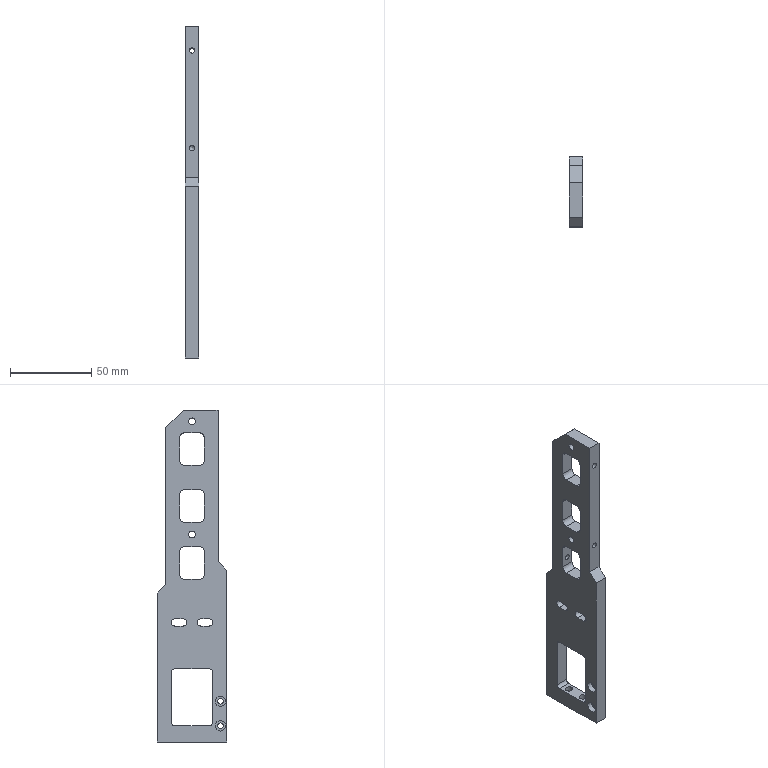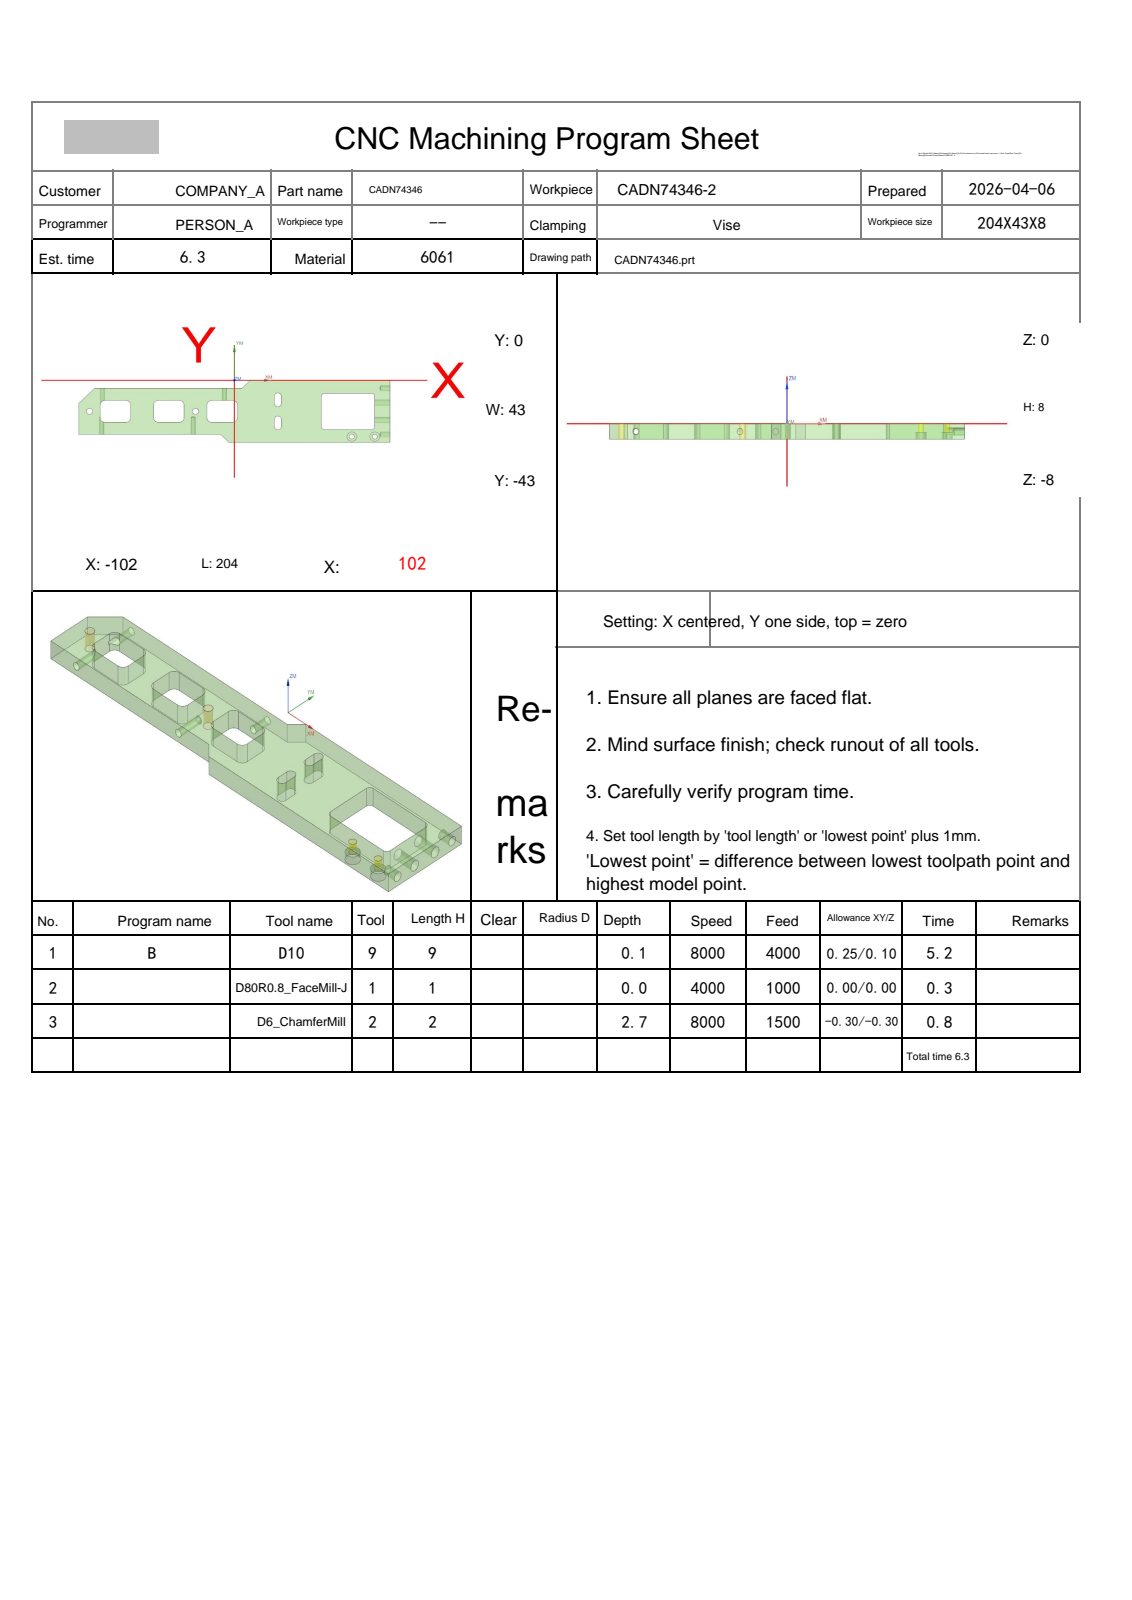NC program | NX | posted by the shop | part box 8 x 43 x 204 mm
Whole program:
%
O0001
(Machine time: 6.90 MIN)
(===Total Tool:3===)
(T9=D10     D=10.  R=0.   D-  H09 Z=0.1   )
(T1=D80R0.8 FaceMill-J D=80.  R=0.8  D-  H01 Z=0.    )
(T2=D6_ChamferMill   D=6.   R=0.   D-  H02 Z=-2.7  )
G80 G90 G17 G49 G40
G91 G28 Z0
M01
N1 T09 M06
(D10  D=10. R=0. H=09 ce=0.25 di=0.10)
G00 G90 G54 X-115.945 Y-22.484 M03 S8000
G43 H09 Z20.
M08
Z2.1
G01 X-115.846 Y-22.469 Z1.476 F4000.
X-115.747 Y-22.454 Z1.228
X-115.648 Y-22.439 Z1.046
X-115.549 Y-22.424 Z.9
X-115.45 Y-22.409 Z.777
X-115.351 Y-22.394 Z.672
X-115.252 Y-22.379 Z.58
X-115.154 Y-22.364 Z.5
X-115.055 Y-22.349 Z.43
X-114.956 Y-22.334 Z.368
X-114.857 Y-22.319 Z.314
X-114.758 Y-22.304 Z.267
X-114.659 Y-22.289 Z.227
X-114.56 Y-22.274 Z.192
X-114.462 Y-22.259 Z.164
X-114.363 Y-22.244 Z.14
X-114.264 Y-22.229 Z.123
X-114.165 Y-22.214 Z.11
X-114.066 Y-22.199 Z.103
X-113.967 Y-22.184 Z.1
X-111.744 Y-21.846
G03 X-111.332 Y-21.478 I-.079 J.502
X-110.863 Y-17.555 I-16.172 J3.923
X-110.865 Y-17.31 I-16.641 J0.0
X-110.777 Y-4.262 I-964.212 J13.048
X-110.784 Y-.447 I-964.301 J0.0
G02 X-105.871 Y6.277 I7.08 J-.016
X-100.069 Y7.207 I5.928 J-18.425
X-91.117 Y7.309 I8.952 J-392.128
X-88.92 Y7.303 I0.0 J-392.231
G01 X103.117 Y7.283
G02 X109.797 Y2.311 I-.087 J-7.089
X110.703 Y-3.395 I-18.567 J-5.872
X110.807 Y-12.349 I-384.71 J-8.954
X110.801 Y-14.594 I-384.814 J0.0
G01 X110.782 Y-42.608
G02 X105.819 Y-49.293 I-7.091 J.079
X100.062 Y-50.204 I-5.895 J18.612
X91.09 Y-50.306 I-8.972 J395.249
X88.914 Y-50.3 I0.0 J395.351
G01 X-103.206 Y-50.279
G02 X-109.795 Y-45.322 I.167 J7.081
X-110.706 Y-39.565 I18.625 J5.895
X-110.813 Y-29.529 I469.253 J10.036
X-110.769 Y-23.117 I469.361 J0.0
G03 X-110.287 Y-11.341 I-143.632 J11.776
X-110.302 Y-9.245 I-144.114 J0.0
G02 X-110.321 Y-6.601 I192.195 J2.644
X-110.247 Y-1.299 I192.213 J0.0
X-105.72 Y5.141 I7.749 J-.636
X-99.729 Y6.584 I6.779 J-14.997
X-91.153 Y6.82 I8.576 J-155.336
X-88.733 Y6.801 I0.0 J-155.573
G01 X101.703 Y6.781
G02 X108.732 Y2.029 I-.178 J-7.838
X110.114 Y-4.183 I-16.043 J-6.827
X110.322 Y-13.597 I-212.824 J-9.414
X110.3 Y-16.63 I-213.032 J0.0
G01 X110.279 Y-41.207
G02 X105.478 Y-48.255 I-7.852 J.19
X99.262 Y-49.617 I-6.818 J16.26
X89.848 Y-49.821 I-9.414 J217.146
X86.815 Y-49.8 I0.0 J217.35
G01 X-101.606 Y-49.785
G02 X-108.755 Y-44.984 I.09 J7.858
X-110.118 Y-38.767 I16.253 J6.82
X-110.322 Y-29.704 I201.613 J9.063
X-110.208 Y-22.923 I201.817 J0.0
G03 X-109.792 Y-9.804 I-206.855 J13.119
X-109.802 Y-7.745 I-207.27 J0.0
G02 X-109.824 Y-6.102 I63.015 J1.643
X-109.706 Y-2.25 I63.036 J0.0
X-104.504 Y4.619 I8.585 J-1.097
X-98.099 Y6.077 I7.273 J-17.164
X-90. Y6.307 I8.099 J-142.165
X-88.454 Y6.299 I0.0 J-142.396
G01 X100.196 Y6.285
G02 X108.151 Y.934 I-.073 J-8.697
X109.589 Y-5.58 I-17.614 J-7.304
X109.814 Y-14.426 I-173.345 J-8.846
X109.799 Y-16.726 I-173.571 J0.0
G01 X109.779 Y-39.808
G02 X104.513 Y-47.613 I-8.667 J.169
X97.912 Y-49.088 I-7.36 J17.422
X88.463 Y-49.319 I-9.449 J193.324
X85.666 Y-49.299 I0.0 J193.555
G01 X-100.306 Y-49.281
G02 X-108.099 Y-44.047 I.16 J8.657
X-109.575 Y-37.6 I17.063 J7.301
X-109.801 Y-28.976 I164.479 J8.624
X-109.469 Y-18.522 I164.705 J0.0
G03 X-109.271 Y-4.345 I-632.065 J15.909
G02 X-103.505 Y4.066 I9.35 J-.227
X-96.604 Y5.579 I7.746 J-18.849
X-86.827 Y5.821 I9.777 J-196.915
X-84.008 Y5.801 I0.0 J-197.157
G01 X99.003 Y5.779
G02 X107.618 Y-.112 I-.099 J-9.389
X109.09 Y-7.074 I-19.438 J-7.747
X109.318 Y-16.758 I-205.596 J-9.684
X109.299 Y-19.52 I-205.824 J0.0
G01 X109.28 Y-38.419
G02 X103.46 Y-47.084 I-9.38 J.014
X96.605 Y-48.576 I-7.719 J18.972
X86.65 Y-48.82 I-9.955 J202.743
X83.709 Y-48.799 I0.0 J202.987
G01 X-98.891 Y-48.783
X-98.896
G02 X-107.63 Y-42.861 I0.0 J9.403
X-109.082 Y-36.048 I19.286 J7.67
X-109.279 Y-28.312 I151.469 J7.736
X-108.994 Y-19.026 I151.666 J0.0
G03 X-108.774 Y-5.638 I-565.816 J16.032
G02 X-102.398 Y3.604 I9.98 J-.065
X-95.281 Y5.079 I8.013 J-20.758
X-85.739 Y5.315 I9.542 J-192.722
X-83.335 Y5.3 I0.0 J-192.958
G01 X97.753 Y5.277
X97.79
G02 X107.101 Y-1.099 I0.0 J-9.987
X108.57 Y-8.117 I-20.6 J-7.972
X108.819 Y-18.212 I-203.774 J-10.095
X108.799 Y-21.112 I-204.024 J0.0
X108.819 Y-27.156 I-890.849 J-6.044
X108.758 Y-37.611 I-890.87 J0.0
X102.551 Y-46.534 I-9.917 J.278
X95.447 Y-48.064 I-8.043 J20.098
X85.798 Y-48.314 I-9.649 J185.638
X83.301 Y-48.298 I0.0 J185.888
G01 X-97.698 Y-48.279
X-97.787 Y-48.28
G02 X-107.099 Y-41.909 I0.0 J9.991
X-108.566 Y-34.941 I20.485 J7.952
X-108.758 Y-27.668 I137.608 J7.273
X-108.515 Y-19.481 I137.801 J0.0
G03 X-108.264 Y-6.575 I-846.193 J22.863
G02 X-101.588 Y3.043 I10.452 J-.129
X-94.173 Y4.572 I8.344 J-21.726
X-84.031 Y4.818 I10.141 J-208.429
X-81.277 Y4.8 I0.0 J-208.676
G01 X96.503 Y4.778
X96.63 Y4.779
G02 X103.222 Y2.577 I0.0 J-10.966
X107.199 Y-3.801 I-7.775 J-9.277
X108.202 Y-11.921 I-33.911 J-8.307
X108.318 Y-26.201 I-876.101 J-14.28
X108.258 Y-36.419 I-876.217 J0.0
X101.735 Y-45.976 I-10.419 J.107
X94.385 Y-47.553 I-8.344 J20.974
X84.097 Y-47.818 I-10.288 J199.468
X81.24 Y-47.798 I0.0 J199.733
G01 X-96.36 Y-47.783
X-96.559 Y-47.785
G02 X-102.827 Y-45.875 I0.0 J11.243
X-107.081 Y-39.603 I7.046 J9.358
X-108.166 Y-32. I29.686 J8.114
X-108.226 Y-27.554 I164.845 J4.446
X-107.991 Y-18.752 I164.905 J0.0
G03 X-107.766 Y-7.612 I-938.507 J24.515
G02 X-104.99 Y-.382 I11.151 J-.133
X-98.283 Y3.32 I9.451 J-9.197
X-90.297 Y4.206 I8.285 J-38.236
X-79.414 Y4.302 I10.883 J-613.879
X-77.848 Y4.3 I0.0 J-613.975
G01 X95.403 Y4.276
X95.537 Y4.277
G02 X101.868 Y2.465 I0.0 J-11.966
X106.449 Y-3.924 I-6.808 J-9.717
X107.646 Y-11.76 I-29.039 J-8.448
X107.813 Y-22.643 I-355.871 J-10.883
X107.799 Y-25.808 I-356.037 J0.0
X107.821 Y-29.207 I-263.412 J-3.399
X107.744 Y-35.557 I-263.434 J0.0
X104.286 Y-43.312 I-10.873 J.2
X97.372 Y-46.521 I-9.282 J10.943
X89.065 Y-47.237 I-8.306 J47.865
G01 X89.063
G02 X79.747 Y-47.302 I-9.316 J666.934
X77.563 Y-47.298 I0.0 J666.999
G01 X-95.186 Y-47.282
G02 X-95.418 Y-47.285 I-.232 J12.483
X-101.385 Y-45.767 I0.0 J12.485
X-106.377 Y-39.294 I6.103 J9.868
X-107.639 Y-31.319 I27.905 J8.505
X-107.702 Y-26.933 I154.715 J4.386
X-107.504 Y-19.107 I154.778 J0.0
G01 X-107.27 Y-8.598
G02 X-104.913 Y-1.646 I11.914 J-.164
X-98.244 Y2.585 I9.847 J-8.15
X-90.086 Y3.673 I8.639 J-33.65
X-79.089 Y3.809 I10.997 J-442.591
X-76.237 Y3.8 I0.0 J-442.727
G01 X94.303 Y3.776
X94.462 Y3.777
G02 X100.602 Y2.248 I0.0 J-13.096
X105.785 Y-4.328 I-6.124 J-10.157
X107.1 Y-11.993 I-27.039 J-8.584
X107.321 Y-23.689 I-309.996 J-11.697
X107.298 Y-27.39 I-310.216 J0.0
X107.322 Y-29.721 I-117.228 J-2.331
X107.194 Y-35.187 I-117.251 J0.0
X100.145 Y-44.906 I-11.124 J.653
X92.651 Y-46.519 I-8.721 J22.3
X83.172 Y-46.803 I-9.479 J158.048
X81.457 Y-46.794 I0.0 J158.332
G01 X-94.043 Y-46.783
G02 X-94.325 Y-46.786 I-.282 J13.724
X-100.241 Y-45.446 I0.0 J13.727
X-105.737 Y-38.809 I5.633 J10.259
X-107.094 Y-30.953 I26.291 J8.587
X-107.173 Y-26.12 I148.356 J4.833
X-106.998 Y-18.917 I148.434 J0.0
X-106.746 Y-9.085 I504.328 J-8.014
X-103.763 Y-1.618 I11.9 J-.424
X-96.742 Y2.254 I9.94 J-9.723
X-87.961 Y3.21 I8.935 J-41.29
X-76.843 Y3.302 I11.117 J-669.755
X-75.211 Y3.3 I0.0 J-669.848
G01 X93.153 Y3.278
G02 X93.39 Y3.28 I.236 J-14.408
X99.412 Y1.961 I0.0 J-14.41
X105.109 Y-4.686 I-5.542 J-10.516
X106.548 Y-12.224 I-25.324 J-8.74
X106.811 Y-22.593 I-204.557 J-10.368
X106.796 Y-25.019 I-204.82 J0.0
X106.818 Y-27.831 I-180.192 J-2.812
X106.714 Y-33.968 I-180.214 J0.0
X103.608 Y-41.535 I-11.728 J.392
X96.679 Y-45.266 I-9.85 J9.996
X88.246 Y-46.198 I-8.754 J40.579
X76.992 Y-46.301 I-11.254 J616.985
X74.997 Y-46.298 I0.0 J617.088
G01 X-93.153 Y-46.278
G02 X-93.389 Y-46.28 I-.236 J14.417
X-99.414 Y-44.961 I0.0 J14.419
X-105.144 Y-38.222 I5.567 J10.54
X-106.577 Y-29.977 I26.255 J8.81
X-106.639 Y-25.462 I166.156 J4.514
X-106.475 Y-18.082 I166.217 J0.0
X-106.227 Y-9.675 I204.317 J-1.806
X-102.959 Y-2.002 I12.08 J-.613
X-95.93 Y1.745 I10.032 J-10.353
X-87.448 Y2.693 I8.89 J-41.107
X-76.093 Y2.804 I11.355 J-581.767
X-73.799 Y2.799 I0.0 J-581.878
G01 X92.253 Y2.775
G02 X92.473 Y2.776 I.219 J-15.102
X98.664 Y1.449 I0.0 J-15.104
X104.556 Y-5.352 I-5.563 J-10.773
X106.048 Y-13.182 I-25.937 J-8.998
X106.306 Y-23.367 I-200.328 J-10.185
X106.295 Y-25.478 I-200.587 J0.0
X106.319 Y-27.822 I-116.062 J-2.344
X106.186 Y-33.375 I-116.086 J0.0
X102.518 Y-41.415 I-11.865 J.557
X95.322 Y-44.882 I-9.94 J11.429
X86.228 Y-45.726 I-9.093 J48.591
G01 X86.223
G02 X76.2 Y-45.8 I-10.023 J672.774
X74.174 Y-45.797 I0.0 J672.848
G01 X-92.156 Y-45.777
G02 X-92.396 Y-45.779 I-.24 J15.585
X-98.35 Y-44.598 I0.0 J15.586
X-104.491 Y-37.817 I5.151 J10.838
X-106.012 Y-29.892 I24.508 J8.81
X-106.12 Y-24.854 I117.66 J5.038
X-106.035 Y-20.395 I117.768 J0.0
X-105.759 Y-10.815 I361.761 J-5.624
X-103.332 Y-3.715 I13.088 J-.51
X-96.287 Y.925 I10.558 J-8.361
X-87.995 Y2.131 I9.103 J-33.474
X-76.166 Y2.315 I11.829 J-380.451
X-72.697 Y2.299 I0.0 J-380.635
G01 X91.103 Y2.279
G02 X91.4 Y2.281 I.297 J-16.894
X97.37 Y1.192 I0.0 J-16.896
X103.908 Y-5.751 I-4.874 J-11.14
X105.518 Y-13.709 I-25.2 J-9.241
X105.811 Y-24.527 I-199.541 J-10.819
X105.795 Y-27.053 I-199.834 J0.0
X105.818 Y-28.559 I-49.572 J-1.506
X105.562 Y-33.593 I-49.595 J0.0
X98.008 Y-43.3 I-11.88 J1.453
X90.171 Y-44.987 I-9.246 J23.908
X80.266 Y-45.3 I-9.905 J156.803
X78.628 Y-45.291 I0.0 J157.115
G01 X-91.056 Y-45.28
G02 X-91.369 Y-45.283 I-.313 J17.11
X-97.281 Y-44.229 I0.0 J17.113
X-103.895 Y-37.281 I4.762 J11.156
X-105.489 Y-29.02 I24.476 J9.008
X-105.582 Y-23.553 I161.068 J5.467
X-105.449 Y-16.999 I161.16 J0.0
X-105.45 Y-16.562 I59.526 J.437
X-105.111 Y-10.216 I59.527 J0.0
X-97.278 Y-.2 I12.22 J-1.486
X-89.435 Y1.478 I9.348 J-24.523
X-79.327 Y1.802 I10.108 J-157.379
X-77.642 Y1.793 I0.0 J-157.704
G01 X89.957 Y1.783
G02 X90.357 Y1.787 I.399 J-18.721
X96.302 Y.818 I0.0 J-18.726
X103.3 Y-6.239 I-4.473 J-11.434
X104.99 Y-14.232 I-24.754 J-9.406
X105.312 Y-25.308 I-189.975 J-11.076
X105.293 Y-28.026 I-190.297 J0.0
X105.309 Y-28.953 I-26.847 J-.928
X104.754 Y-34.387 I-26.863 J0.0
X97.529 Y-42.685 I-11.757 J2.942
X89.609 Y-44.46 I-9.435 J23.541
X79.639 Y-44.797 I-9.97 J147.09
X78.117 Y-44.789 I0.0 J147.428
G01 X-90.333 Y-44.774
G02 X-90.575 Y-44.776 I-.242 J17.401
X-96.651 Y-43.681 I0.0 J17.402
X-103.358 Y-36.613 I4.874 J11.342
X-104.944 Y-28.55 I24.275 J8.96
X-105.061 Y-23.103 I126.284 J5.447
X-104.986 Y-18.753 I126.401 J0.0
G01 Y-18.574
G02 X-104.668 Y-11.361 I81.884 J0.0
X-96.56 Y-.706 I12.548 J-1.136
X-88.416 Y.991 I9.564 J-25.512
X-77.377 Y1.312 I11.04 J-189.877
X-74.923 Y1.296 I0.0 J-190.197
G01 X89.077 Y1.281
G02 X89.479 Y1.285 I.402 J-19.649
X95.526 Y.332 I0.0 J-19.653
X102.695 Y-6.721 I-4.382 J-11.624
X104.452 Y-14.644 I-24.164 J-9.513
X104.803 Y-24.804 I-146.731 J-10.16
X104.681 Y-30.784 I-147.082 J0.0
X102.1 Y-38.189 I-13.435 J.531
X94.945 Y-42.861 I-10.828 J8.769
X86.159 Y-44.129 I-9.542 J35.023
X74.509 Y-44.309 I-11.65 J377.282
X71.361 Y-44.296 I0.0 J377.462
G01 X-89.089 Y-44.281
G02 X-89.485 Y-44.285 I-.396 J19.654
X-95.49 Y-43.345 I0.0 J19.658
X-102.767 Y-36.097 I4.359 J11.652
X-104.413 Y-27.847 I24.245 J9.128
X-104.54 Y-21.894 I139.916 J5.952
X-104.231 Y-12.606 I140.043 J0.0
X-101.318 Y-5.075 I13.553 J-.913
X-94.103 Y-.601 I10.9 J-9.525
X-85.259 Y.633 I9.615 J-36.583
X-73.188 Y.812 I12.072 J-407.399
X-69.811 Y.798 I0.0 J-407.578
G01 X88.388 Y.777
G02 X88.706 Y.779 I.317 J-20.105
X94.791 Y-.163 I0.0 J-20.107
X102.235 Y-7.53 I-4.384 J-11.875
X103.96 Y-15.566 I-25.223 J-9.617
X104.293 Y-24.523 I-120.082 J-8.957
X104.159 Y-30.205 I-120.416 J0.0
X101.389 Y-37.791 I-13.502 J.632
X94.037 Y-42.411 I-10.961 J9.285
X85.192 Y-43.634 I-9.599 J36.826
X73.649 Y-43.807 I-11.543 J385.533
X70.744 Y-43.796 I0.0 J385.706
G01 X-88.456 Y-43.775
G02 X-88.773 Y-43.778 I-.318 J19.56
X-94.995 Y-42.762 I0.0 J19.563
X-102.242 Y-35.426 I4.578 J11.77
X-103.891 Y-27.023 I24.762 J9.221
X-104.023 Y-21.49 I115.429 J5.533
X-103.731 Y-13.283 I115.562 J0.0
X-100.757 Y-5.645 I13.787 J-.971
X-93.45 Y-1.122 I11.042 J-9.676
X-84.509 Y.129 I9.74 J-37.034
X-72.177 Y.313 I12.331 J-412.319
X-68.611 Y.298 I0.0 J-412.504
G01 X87.639 Y.274
G02 X87.948 Y.276 I.31 J-20.366
X94.235 Y-.718 I0.0 J-20.368
X101.69 Y-8.125 I-4.527 J-12.012
X103.466 Y-16.459 I-25.763 J-9.847
X103.774 Y-24.419 I-102.896 J-7.96
X103.651 Y-29.448 I-103.203 J0.0
X101.069 Y-36.903 I-13.911 J.644
X93.756 Y-41.776 I-11.153 J8.814
X84.929 Y-43.106 I-9.746 J34.744
X72.875 Y-43.311 I-12.054 J353.277
X69.532 Y-43.295 I0.0 J353.483
G01 X-87.618 Y-43.274
G02 X-87.943 Y-43.277 I-.325 J20.369
X-94.261 Y-42.272 I0.0 J20.372
X-101.731 Y-34.734 I4.536 J11.966
X-103.359 Y-26.377 I25.127 J9.232
X-103.506 Y-21.163 I92.478 J5.214
X-103.212 Y-13.788 I92.625 J0.0
X-99.982 Y-5.955 I13.775 J-1.098
X-92.439 Y-1.537 I11.144 J-10.377
X-83.335 Y-.356 I9.827 J-40.076
X-71.744 Y-.194 I11.59 J-416.177
X-69.086 Y-.203 I0.0 J-416.338
G01 X86.614 Y-.223
G02 X87.007 Y-.219 I.393 J-22.059
X93.323 Y-1.143 I0.0 J-22.062
X101.124 Y-8.657 I-4.263 J-12.233
X102.912 Y-16.632 I-24.987 J-9.789
X103.253 Y-24.25 I-84.963 J-7.618
X103.128 Y-28.869 I-85.304 J0.0
X100.335 Y-36.561 I-13.927 J.705
X92.992 Y-41.293 I-11.197 J9.31
X84.061 Y-42.608 I-9.847 J35.893
X72.082 Y-42.81 I-11.979 J355.775
X68.863 Y-42.795 I0.0 J355.976
G01 X-86.686 Y-42.775
G02 X-87.051 Y-42.779 I-.365 J21.742
X-93.392 Y-41.834 I0.0 J21.745
X-101.136 Y-34.258 I4.301 J12.143
X-102.818 Y-25.912 I24.758 J9.331
X-102.981 Y-20.92 I76.442 J4.992
X-102.701 Y-14.374 I76.605 J0.0
X-99.258 Y-6.327 I13.841 J-1.162
X-91.667 Y-2.017 I11.198 J-10.884
X-82.459 Y-.853 I9.923 J-41.485
X-70.035 Y-.691 I12.425 J-475.745
X-66.661 Y-.703 I0.0 J-475.907
G01 X85.839 Y-.725
G02 X86.206 Y-.722 I.367 J-23.009
X92.506 Y-1.601 I0.0 J-23.012
X100.586 Y-9.243 I-4.107 J-12.435
X102.426 Y-17.557 I-25.584 J-10.023
X102.728 Y-24.026 I-69.282 J-6.468
X102.587 Y-28.445 I-69.584 J0.0
X99.409 Y-36.438 I-13.756 J.841
X91.966 Y-40.89 I-11.184 J10.252
X83.02 Y-42.119 I-9.854 J38.523
X71.158 Y-42.306 I-11.862 J376.211
X68.172 Y-42.295 I0.0 J376.398
G01 X-85.578 Y-42.28
G02 X-86.047 Y-42.285 I-.47 J24.225
X-92.305 Y-41.462 I0.0 J24.23
X-100.615 Y-33.609 I3.87 J12.419
X-102.287 Y-25.311 I25.04 J9.361
X-102.454 Y-20.773 I61.578 J4.538
X-102.157 Y-14.725 I61.745 J0.0
X-98.168 Y-6.335 I13.651 J-1.346
X-90.601 Y-2.42 I11.083 J-12.152
X-81.23 Y-1.336 I9.996 J-45.368
X-69.474 Y-1.198 I11.756 J-500.016
X-67.181 Y-1.203 I0.0 J-500.155
G01 X84.969 Y-1.224
G02 X85.384 Y-1.22 I.415 J-24.055
X91.79 Y-2.089 I0.0 J-24.059
X100.009 Y-9.728 I-4.034 J-12.581
X101.9 Y-18.029 I-25.245 J-10.118
X102.196 Y-23.805 I-56.222 J-5.776
X102.032 Y-28.115 I-56.517 J0.0
X98.125 Y-36.645 I-13.482 J1.016
X90.418 Y-40.614 I-11.1 J12.085
X81.043 Y-41.668 I-9.964 J46.437
X68.687 Y-41.802 I-12.356 J566.888
X65.744 Y-41.795 I0.0 J567.022
G01 X-85.106 Y-41.773
G02 X-85.454 Y-41.776 I-.348 J23.598
X-91.825 Y-40.9 I0.0 J23.6
X-100.054 Y-33.066 I4.041 J12.485
X-101.749 Y-24.824 I24.934 J9.423
X-101.921 Y-20.694 I49.685 J4.13
X-101.593 Y-14.991 I49.856 J0.0
X-93.009 Y-3.926 I13.495 J-1.607
X-84.49 Y-2.074 I10.256 J-26.657
X-73.581 Y-1.704 I10.909 J-160.357
X-71.948 Y-1.712 I0.0 J-160.728
G01 X84.352 Y-1.728
G02 X84.702 Y-1.725 I.35 J-24.212
X91.172 Y-2.605 I0.0 J-24.215
X99.517 Y-10.404 I-4.081 J-12.732
X101.381 Y-18.567 I-25.436 J-10.101
X101.657 Y-23.6 I-45.716 J-5.033
X101.46 Y-27.85 I-45.992 J0.0
X92.928 Y-39.085 I-13.352 J1.283
X84.605 Y-40.911 I-10.139 J26.33
X73.496 Y-41.297 I-11.108 J159.508
X71.664 Y-41.287 I0.0 J159.895
G01 X-84.386 Y-41.271
G02 X-84.714 Y-41.274 I-.328 J24.162
X-91.156 Y-40.399 I0.0 J24.164
X-99.57 Y-32.341 I4.044 J12.645
X-101.243 Y-23.89 I25.875 J9.511
X-101.381 Y-20.61 I38.954 J3.279
X-100.978 Y-15.013 I39.091 J0.0
X-92.406 Y-4.444 I13.486 J-2.177
X-83.789 Y-2.577 I10.361 J-26.996
X-72.261 Y-2.197 I11.527 J-174.752
X-70.147 Y-2.209 I0.0 J-175.132
G01 X83.603 Y-2.229
G02 X83.968 Y-2.226 I.366 J-24.7
X90.571 Y-3.125 I0.0 J-24.703
X98.954 Y-10.904 I-4.11 J-12.834
X100.889 Y-19.4 I-25.63 J-10.305
X101.111 Y-23.416 I-36.191 J-4.016
X100.842 Y-27.83 I-36.413 J0.0
X92.581 Y-38.455 I-13.284 J1.805
X84.034 Y-40.396 I-10.354 J25.802
X72.818 Y-40.796 I-11.216 J157.028
X70.994 Y-40.786 I0.0 J157.428
G01 X-83.406 Y-40.775
G02 X-83.796 Y-40.778 I-.39 J26.314
X-90.191 Y-39.989 I0.0 J26.317
X-98.978 Y-31.891 I3.69 J12.821
X-100.705 Y-23.403 I25.434 J9.593
X-100.829 Y-20.593 I31.714 J2.81
X-100.341 Y-15.035 I31.839 J0.0
X-92.131 Y-5.099 I13.378 J-2.693
X-83.743 Y-3.139 I10.391 J-25.541
X-72.616 Y-2.707 I11.127 J-143.09
X-71.054 Y-2.715 I0.0 J-143.522
G01 X82.596 Y-2.725
G02 X83.055 Y-2.721 I.459 J-26.788
X89.676 Y-3.552 I0.0 J-26.792
X98.477 Y-11.597 I-3.867 J-13.067
X100.406 Y-20.401 I-26.307 J-10.376
X100.56 Y-23.304 I-27.247 J-2.903
X100.088 Y-28.366 I-27.402 J0.0
X92.025 Y-37.917 I-13.114 J2.892
X83.583 Y-39.871 I-10.379 J25.627
X72.126 Y-40.298 I-11.457 J153.741
X70.194 Y-40.285 I0.0 J154.168
G01 X-82.756 Y-40.272
G02 X-83.149 Y-40.275 I-.393 J26.075
X-89.733 Y-39.43 I0.0 J26.078
X-98.427 Y-31.347 I3.864 J12.873
X-100.184 Y-22.56 I25.457 J9.659
X-100.268 Y-20.509 I24.867 J2.051
X-99.551 Y-14.571 I24.952 J0.0
X-91.48 Y-5.59 I13.196 J-3.742
X-82.933 Y-3.628 I10.502 J-26.16
X-71.526 Y-3.203 I11.407 J-152.975
X-69.744 Y-3.214 I0.0 J-153.4
G01 X82.056 Y-3.229
G02 X82.444 Y-3.226 I.388 J-26.547
X89.132 Y-4.082 I0.0 J-26.55
X97.906 Y-12.067 I-3.933 J-13.135
X99.892 Y-21.21 I-25.759 J-10.382
X99.99 Y-23.273 I-21.647 J-2.063
X99.252 Y-28.892 I-21.745 J0.0
X91.431 Y-37.399 I-12.901 J4.013
X83.041 Y-39.355 I-10.409 J25.669
X71.723 Y-39.792 I-11.317 J146.323
X70.052 Y-39.783 I0.0 J146.76
G01 X-81.848 Y-39.775
G02 X-82.274 Y-39.778 I-.426 J28.169
X-88.788 Y-39.014 I0.0 J28.172
X-97.86 Y-30.846 I3.536 J13.051
X-99.657 Y-21.314 I25.206 J9.685
X-99.685 Y-20.268 I19.118 J1.046
X-98.472 Y-13.56 I19.147 J0.0
X-90.824 Y-6.076 I12.788 J-5.419
X-82.228 Y-4.127 I10.558 J-26.639
X-71.032 Y-3.709 I11.196 J-149.734
X-69.538 Y-3.716 I0.0 J-150.152
G01 X81.112 Y-3.726
G02 X81.552 Y-3.722 I.44 J-28.877
X88.152 Y-4.487 I0.0 J-28.88
X97.453 Y-12.801 I-3.602 J-13.389
X99.371 Y-22.795 I-25.086 J-9.994
X99.102 Y-26.596 I-27.003 J0.0
X91.137 Y-36.748 I-13.267 J2.209
X82.624 Y-38.827 I-10.576 J24.832
X71.025 Y-39.294 I-11.599 J143.915
X69.237 Y-39.283 I0.0 J144.382
G01 X-81.063 Y-39.275
G02 X-81.526 Y-39.279 I-.463 J29.052
X-88.105 Y-38.524 I0.0 J29.056
X-97.375 Y-30.155 I3.497 J13.191
X-99.073 Y-21.061 I23.494 J9.094
X-98.664 Y-16.54 I25.193 J0.0
X-90.638 Y-6.768 I13.407 J-2.831
X-82.176 Y-4.69 I10.637 J-25.052
X-71.311 Y-4.222 I10.866 J-125.781
X-70.39 Y-4.225 I0.0 J-126.25
G01 X80.36 Y-4.226
G02 X80.83 Y-4.222 I.47 J-29.55
X87.55 Y-4.996 I0.0 J-29.553
X96.849 Y-13.179 I-3.578 J-13.441
X98.761 Y-22.624 I-22.362 J-9.445
X98.487 Y-26.262 I-24.275 J0.0
X90.697 Y-36.161 I-13.194 J2.369
X82.199 Y-38.299 I-10.645 J24.344
X70.904 Y-38.785 I-11.295 J131.172
X69.513 Y-38.777 I0.0 J131.658
G01 X-80.237 Y-38.776
G02 X-80.755 Y-38.78 I-.518 J30.176
X-87.431 Y-38.033 I0.0 J30.181
X-96.855 Y-29.55 I3.445 J13.304
X-98.456 Y-21.15 I21.238 J8.4
X-98.071 Y-16.972 I22.839 J0.0
X-90.086 Y-7.297 I13.366 J-2.898
X-81.578 Y-5.198 I10.706 J-25.108
X-70.628 Y-4.723 I10.95 J-125.81
X-69.692 Y-4.726 I0.0 J-126.285
G01 X79.607
G02 X80.091 Y-4.722 I.483 J-30.609
X86.85 Y-5.477 I0.0 J-30.613
X96.367 Y-13.838 I-3.504 J-13.586
X98.134 Y-22.478 I-20.242 J-8.64
X97.876 Y-25.837 I-22.009 J0.0
X90.229 Y-35.587 I-13.117 J2.414
X81.836 Y-37.765 I-10.668 J23.85
X70.553 Y-38.28 I-11.283 J123.147
X69.302 Y-38.274 I0.0 J123.663
G01 X-79.847 Y-38.27
G02 X-80.272 Y-38.273 I-.424 J28.761
X-87.081 Y-37.455 I0.0 J28.764
X-96.283 Y-29.076 I3.688 J13.292
X-97.823 Y-21.272 I19.008 J7.804
X-97.406 Y-17.154 I20.548 J0.0
X-89.707 Y-7.906 I13.203 J-3.164
X-81.317 Y-5.743 I10.735 J-24.281
X-69.685 Y-5.214 I11.632 J-127.635
X-68.234 Y-5.222 I0.0 J-128.164
G01 X79.166 Y-5.23
G02 X79.55 Y-5.228 I.383 J-29.911
X86.356 Y-6.013 I0.0 J-29.914
X95.906 Y-14.548 I-3.621 J-13.663
X97.489 Y-22.3 I-18.193 J-7.752
X97.2 Y-25.669 I-19.775 J0.0
X89.774 Y-35.005 I-12.962 J2.688
X81.153 Y-37.266 I-10.832 J23.736
X69.993 Y-37.776 I-11.16 J121.841
X68.919 Y-37.771 I0.0 J122.351
G01 X-79.131 Y-37.77
G02 X-79.55 Y-37.773 I-.419 J29.668
X-86.369 Y-36.978 I0.0 J29.671
X-95.781 Y-28.429 I3.584 J13.4
X-97.169 Y-21.391 I17.138 J7.038
X-96.711 Y-17.293 I18.527 J0.0
X-89.326 Y-8.518 I13.006 J-3.45
X-80.708 Y-6.248 I10.91 J-23.926
X-69.445 Y-5.724 I11.263 J-120.649
X-68.424 Y-5.728 I0.0 J-121.173
G01 X78.476 Y-5.731
G02 X78.902 Y-5.728 I.426 J-29.932
X85.91 Y-6.56 I0.0 J-29.935
X95.447 Y-15.273 I-3.775 J-13.708
X96.824 Y-22.119 I-16.332 J-6.846
X96.464 Y-25.669 I-17.709 J0.0
X89.181 Y-34.491 I-12.779 J3.133
X80.616 Y-36.752 I-10.828 J23.669
X69.501 Y-37.272 I-11.115 J118.478
X68.582 Y-37.268 I0.0 J118.998
G01 X-78.367 Y-37.27
G02 X-78.833 Y-37.274 I-.466 J30.412
X-85.755 Y-36.476 I0.0 J30.416
X-95.365 Y-27.539 I3.587 J13.493
X-96.496 Y-21.516 I15.471 J6.024
X-95.933 Y-17.228 I16.602 J0.0
X-88.826 Y-9.074 I12.761 J-3.949
X-80.367 Y-6.785 I10.882 J-23.439
X-68.825 Y-6.222 I11.542 J-118.011
X-67.636 Y-6.228 I0.0 J-118.574
G01 X77.664 Y-6.23
G02 X78.134 Y-6.226 I.47 J-31.373
X85.153 Y-7.021 I0.0 J-31.376
X95.012 Y-16.088 I-3.598 J-13.807
X96.138 Y-21.939 I-14.636 J-5.851
X95.632 Y-25.903 I-15.762 J0.0
X88.772 Y-33.882 I-12.48 J3.791
X80.428 Y-36.195 I-10.792 J22.729
X69.135 Y-36.769 I-11.293 J110.753
X68.198 Y-36.765 I0.0 J111.327
G01 X-76.302 Y-36.785
G02 X-77.19 Y-36.795 I-.888 J42.299
X-83.923 Y-36.256 I0.0 J42.308
X-95.012 Y-26.393 I2.398 J13.862
X-95.806 Y-21.641 I13.828 J4.752
X-94.869 Y-16.493 I14.622 J0.0
X-87.743 Y-9.35 I12.462 J-5.307
X-79.19 Y-7.224 I10.831 J-25.305
X-67.557 Y-6.717 I11.633 J-133.2
X-66.205 Y-6.724 I0.0 J-133.707
G01 X76.995 Y-6.73
G02 X77.459 Y-6.727 I.464 J-32.064
X84.487 Y-7.507 I0.0 J-32.067
X94.68 Y-17.279 I-3.501 J-13.854
X95.436 Y-21.774 I-12.999 J-4.495
X94.4 Y-27.011 I-13.754 J0.0
X87.474 Y-33.705 I-12.135 J5.625
X78.861 Y-35.799 I-10.773 J25.544
X67.698 Y-36.274 I-11.164 J131.047
X66.725 Y-36.271 I0.0 J131.522
G01 X-76.675 Y-36.274
G02 X-77.204 Y-36.278 I-.53 J34.652
X-84.029 Y-35.6 I0.0 J34.656
X-94.719 Y-24.748 I3.033 J13.679
X-95.094 Y-21.685 I12.311 J3.063
X-88.305 Y-10.452 I12.687 J0.0
X-80.079 Y-7.917 I10.958 J-20.945
X-68.906 Y-7.249 I11.173 J-93.078
X-68.456 Y-7.25 I0.0 J-93.746
G01 X-57.456 Y-7.207
X75.993 Y-7.226
G02 X76.541 Y-7.222 I.547 J-35.386
X83.497 Y-7.912 I0.0 J-35.39
X94.664 Y-21.753 I-2.994 J-13.841
X94.451 Y-24.201 I-14.161 J0.0
X88.114 Y-32.559 I-12.143 J2.626
X79.942 Y-35.085 I-10.858 J20.638
X68.779 Y-35.751 I-11.163 J93.232
X68.269 Y-35.75 I0.0 J93.898
G01 X57.619 Y-35.791
X-76.031 Y-35.773
G02 X-76.571 Y-35.778 I-.54 J34.74
X-83.484 Y-35.083 I0.0 J34.744
X-94.292 Y-21.773 I2.793 J13.31
X-94.019 Y-19.066 I13.6 J0.0
X-87.612 Y-10.916 I12.188 J-2.989
X-79.378 Y-8.408 I10.934 J-21.13
X-68.115 Y-7.746 I11.263 J-95.535
X-67.604 Y-7.748 I0.0 J-96.196
G01 X-55.454 Y-7.707
X75.396 Y-7.727
G02 X75.965 Y-7.722 I.57 J-34.808
X83.094 Y-8.46 I0.0 J-34.813
X93.907 Y-21.874 I-2.914 J-13.414
G01 Y-21.945
G02 X88.108 Y-31.678 I-11.844 J.462
X80.265 Y-34.433 I-10.853 J18.357
X69.259 Y-35.225 I-11.006 J76.07
G01 X69.203
X56.604 Y-35.29
X-75.396 Y-35.273
G02 X-75.962 Y-35.277 I-.566 J34.472
X-83.045 Y-34.542 I0.0 J34.477
X-93.482 Y-22.859 I2.836 J13.037
X-93.515 Y-21.975 I11.667 J.884
X-88.103 Y-12.108 I11.701 J0.0
X-80.29 Y-9.16 I10.999 J-17.327
X-69.336 Y-8.288 I11.06 J-69.654
X-58.406 Y-8.204 I10.93 J-712.279
X-55.936 Y-8.208 I0.0 J-712.363
G01 X74.964 Y-8.231
G02 X75.423 Y-8.228 I.459 J-34.507
X82.512 Y-8.964 I0.0 J-34.51
X92.585 Y-18.072 I-2.858 J-13.284
X93.084 Y-21.388 I-10.767 J-3.316
X88.122 Y-30.725 I-11.266 J0.0
X80.315 Y-33.807 I-10.954 J16.323
X69.714 Y-34.7 I-10.874 J65.687
X57.821 Y-34.796 I-11.893 J736.762
X54.914 Y-34.79 I0.0 J736.858
G01 X-74.635 Y-34.773
G02 X-75.196 Y-34.778 I-.56 J36.557
X-82.142 Y-34.112 I0.0 J36.561
X-91.354 Y-27.347 I2.591 J13.182
X-92.676 Y-22.081 I9.826 J5.266
X-87.948 Y-12.967 I11.149 J0.0
X-80.097 Y-9.747 I11.077 J-15.825
X-69.301 Y-8.802 I11.046 J-64.091
X-57.606 Y-8.705 I11.695 J-704.962
X-55.552 Y-8.708 I0.0 J-705.059
G01 X73.998 Y-8.727
G02 X74.586 Y-8.722 I.588 J-36.907
X81.752 Y-9.424 I0.0 J-36.912
X90.783 Y-15.865 I-2.696 J-13.333
X92.231 Y-21.253 I-9.299 J-5.388
X87.97 Y-29.823 I-10.747 J0.0
X80.479 Y-33.137 I-10.888 J14.485
X70.744 Y-34.15 I-10.55 J54.123
X57.957 Y-34.295 I-12.787 J564.969
X55.546 Y-34.29 I0.0 J565.114
G01 X-73.954 Y-34.273
G02 X-74.551 Y-34.278 I-.597 J36.855
X-81.61 Y-33.596 I0.0 J36.859
X-90.104 Y-27.909 I2.593 J13.062
X-91.802 Y-22.17 I8.852 J5.739
X-87.884 Y-13.965 I10.55 J0.0
X-80.572 Y-10.495 I10.923 J-13.576
X-70.903 Y-9.375 I10.636 J-49.53
X-57.371 Y-9.196 I13.532 J-512.296
X-53.854 Y-9.209 I0.0 J-512.474
G01 X73.346 Y-9.227
G02 X73.957 Y-9.222 I.611 J-37.22
X81.198 Y-9.933 I0.0 J-37.225
X89.498 Y-15.313 I-2.674 J-13.217
X91.333 Y-21.148 I-8.358 J-5.835
X87.69 Y-28.957 I-10.193 J0.0
X80.377 Y-32.506 I-10.826 J13.001
X70.557 Y-33.632 I-10.647 J49.456
X57.653 Y-33.797 I-12.905 J505.031
X54.859 Y-33.789 I0.0 J505.196
G01 X-73.291 Y-33.773
G02 X-73.895 Y-33.778 I-.604 J37.456
X-80.997 Y-33.098 I0.0 J37.461
X-88.751 Y-28.423 I2.561 J13.014
X-90.884 Y-22.259 I7.838 J6.164
X-87.597 Y-14.86 I9.971 J0.0
X-80.516 Y-11.15 I10.822 J-12.045
X-71.065 Y-9.911 I10.588 J-44.107
X-57.625 Y-9.695 I13.44 J-416.833
X-54.167 Y-9.709 I0.0 J-417.049
G01 X72.982 Y-9.732
G02 X73.47 Y-9.729 I.488 J-36.357
X80.684 Y-10.451 I0.0 J-36.36
X88.361 Y-15.133 I-2.661 J-13.
X90.387 Y-21.048 I-7.62 J-5.915
X87.258 Y-28.16 I-9.646 J0.0
X80.089 Y-31.906 I-10.721 J11.785
X70.332 Y-33.114 I-10.644 J45.957
X57.223 Y-33.3 I-13.109 J462.563
X54.084 Y-33.289 I0.0 J462.749
G01 X-72.966 Y-33.268
G02 X-73.443 Y-33.271 I-.477 J36.085
X-80.519 Y-32.571 I0.0 J36.088
X-87.775 Y-28.32 I2.551 J12.674
X-89.918 Y-22.347 I7.253 J5.973
X-87.229 Y-15.766 I9.396 J0.0
X-80.358 Y-11.799 I10.681 J-10.567
X-71.226 Y-10.454 I10.464 J-39.374
X-58.478 Y-10.199 I12.747 J-318.147
X-55.729 Y-10.211 I0.0 J-318.402
G01 X71.971 Y-10.227
G02 X72.598 Y-10.222 I.628 J-39.432
X79.829 Y-10.891 I0.0 J-39.437
X86.921 Y-14.702 I-2.477 J-13.114
X89.392 Y-20.943 I-6.646 J-6.241
X86.738 Y-27.373 I-9.117 J0.0
X79.989 Y-31.237 I-10.467 J10.456
X70.854 Y-32.556 I-10.367 J39.501
X57.97 Y-32.801 I-12.885 J339.388
X55.008 Y-32.788 I0.0 J339.632
G01 X-71.992 Y-32.772
G02 X-72.606 Y-32.777 I-.614 J38.594
X-79.75 Y-32.11 I0.0 J38.598
X-86.635 Y-28.352 I2.353 J12.495
X-88.895 Y-22.438 I6.605 J5.914
X-86.59 Y-16.475 I8.866 J0.0
X-79.976 Y-12.4 I10.451 J-9.56
X-71.109 Y-10.987 I10.324 J-36.257
X-58.778 Y-10.703 I12.331 J-267.229
X-56.464 Y-10.713 I0.0 J-267.513
G01 X71.736 Y-10.733
G02 X72.218 Y-10.73 I.482 J-37.3
X79.439 Y-11.436 I0.0 J-37.303
X86.053 Y-15.005 I-2.442 J-12.434
X88.34 Y-20.838 I-6.292 J-5.832
X86.23 Y-26.472 I-8.579 J0.0
X79.797 Y-30.567 I-10.239 J8.984
X71.037 Y-32.005 I-10.194 J34.709
X58.666 Y-32.296 I-12.371 J262.144
X56.242 Y-32.285 I0.0 J262.436
G01 X-71.708 Y-32.267
G02 X-72.195 Y-32.27 I-.487 J36.729
X-79.312 Y-31.574 I0.0 J36.732
X-85.608 Y-28.186 I2.325 J11.862
X-87.809 Y-22.534 I6.155 J5.651
X-85.908 Y-17.229 I8.356 J0.0
X-79.6 Y-13.024 I10.178 J-8.436
X-70.903 Y-11.519 I10.206 J-33.093
X-58.745 Y-11.205 I12.158 J-235.359
X-56.608 Y-11.215 I0.0 J-235.673
G01 X71.042 Y-11.232
G02 X71.539 Y-11.229 I.498 J-38.398
X78.748 Y-11.912 I0.0 J-38.402
X84.904 Y-15.067 I-2.257 J-11.985
X87.215 Y-20.734 I-5.792 J-5.667
X85.396 Y-25.849 I-8.103 J0.0
X79.208 Y-30.002 I-9.958 J8.152
X70.76 Y-31.476 I-9.972 J32.209
X58.037 Y-31.8 I-12.722 J249.334
X55.316 Y-31.785 I0.0 J249.658
G01 X-71.034 Y-31.767
G02 X-71.553 Y-31.771 I-.518 J37.144
X-78.689 Y-31.079 I0.0 J37.147
X-84.503 Y-28.035 I2.16 J11.201
X-86.647 Y-22.632 I5.738 J5.403
X-85.05 Y-17.875 I7.881 J0.0
X-79.086 Y-13.626 I9.832 J-7.49
X-70.605 Y-12.048 I10.029 J-30.325
X-58.61 Y-11.707 I11.995 J-210.712
X-56.612 Y-11.717 I0.0 J-211.053
G01 X69.988 Y-11.727
G02 X70.668 Y-11.722 I.68 J-41.436
X77.95 Y-12.366 I0.0 J-41.442
X83.693 Y-15.144 I-2.007 J-11.478
X86.011 Y-20.626 I-5.325 J-5.482
X84.531 Y-25.146 I-7.642 J0.0
X78.604 Y-29.418 I-9.659 J7.151
X70.621 Y-30.931 I-9.657 J29.141
X58.513 Y-31.294 I-12.108 J202.131
X56.328 Y-31.282 I0.0 J202.494
G01 X-69.972 Y-31.272
G02 X-70.666 Y-31.278 I-.695 J40.163
X-77.832 Y-30.634 I0.0 J40.169
X-83.272 Y-27.935 I1.861 J10.581
X-85.398 Y-22.73 I5.306 J5.205
X-84.059 Y-18.473 I7.433 J0.0
X-78.251 Y-14.137 I9.541 J-6.722
X-70.372 Y-12.588 I9.604 J-28.039
X-58.463 Y-12.209 I11.909 J-186.642
X-56.53 Y-12.219 I0.0 J-187.022
G01 X69.72 Y-12.232
G02 X70.243 Y-12.229 I.523 J-39.879
X77.331 Y-12.864 I0.0 J-39.882
X82.504 Y-15.327 I-1.803 J-10.448
X84.712 Y-20.522 I-5.008 J-5.195
X83.438 Y-24.617 I-7.216 J0.0
X77.768 Y-28.891 I-9.317 J6.461
X69.691 Y-30.444 I-9.559 J27.939
X57.448 Y-30.796 I-12.243 J212.875
X55.048 Y-30.783 I0.0 J213.227
G01 X-69.701 Y-30.767
G02 X-70.212 Y-30.771 I-.511 J38.994
X-77.114 Y-30.155 I0.0 J38.998
X-82.112 Y-27.667 I1.613 J9.503
X-84.044 Y-22.825 I5.101 J4.842
X-82.878 Y-18.945 I7.033 J0.0
X-77.296 Y-14.632 I9.192 J-6.126
X-69.574 Y-13.086 I9.355 J-26.683
X-57.387 Y-12.703 I12.187 J-193.59
X-55.082 Y-12.717 I0.0 J-193.973
G01 X69.068 Y-12.732
G02 X69.622 Y-12.728 I.554 J-40.074
X76.631 Y-13.346 I0.0 J-40.078
X81.443 Y-15.736 I-1.507 J-9.074
X83.298 Y-20.423 I-4.994 J-4.687
X82.141 Y-24.232 I-6.849 J0.0
X76.673 Y-28.43 I-8.983 J6.041
X69.04 Y-29.932 I-9.161 J26.421
X57.819 Y-30.284 I-11.22 J178.412
X56.247 Y-30.277 I0.0 J178.764
G01 X-68.753 Y-30.271
G02 X-69.433 Y-30.277 I-.68 J40.481
X-76.319 Y-29.687 I0.0 J40.487
X-81.007 Y-27.21 I1.316 J8.166
X-82.562 Y-22.914 I5.154 J4.295
X-81.434 Y-19.191 I6.709 J0.0
X-75.959 Y-15.016 I8.879 J-5.967
X-68.072 Y-13.532 I9.208 J-27.235
X-55.903 Y-13.202 I12.169 J-223.766
X-53.428 Y-13.215 I0.0 J-224.097
G01 X68.472 Y-13.233
G02 X69.071 Y-13.228 I.599 J-38.998
X75.935 Y-13.837 I0.0 J-39.003
X80.506 Y-16.485 I-1.235 J-7.401
X81.741 Y-20.326 I-5.358 J-3.841
X80.537 Y-24.124 I-6.593 J0.0
X75.108 Y-28.105 I-8.679 J6.144
X67.352 Y-29.494 I-8.975 J27.76
X55.585 Y-29.794 I-11.767 J230.85
X53.307 Y-29.783 I0.0 J231.15
G01 X-68.443 Y-29.767
G02 X-68.99 Y-29.771 I-.547 J38.443
X-75.461 Y-29.222 I0.0 J38.447
X-80.065 Y-26.237 I1.055 J6.671
X-80.918 Y-23.006 I5.698 J3.232
X-79.573 Y-19.03 I6.55 J0.0
X-74.055 Y-15.245 I8.571 J-6.583
X-66.281 Y-13.97 I8.87 J-29.728
X-54.715 Y-13.706 I11.567 J-253.986
X-52.585 Y-13.715 I0.0 J-254.25
G01 X67.864 Y-13.733
G02 X68.413 Y-13.729 I.548 J-39.572
X74.835 Y-14.254 I0.0 J-39.576
X79.548 Y-17.8 I-.928 J-6.137
X80.001 Y-20.201 I-6.133 J-2.4
X78.364 Y-24.546 I-6.586 J0.0
X72.824 Y-27.959 I-8.362 J7.371
X64.972 Y-29.083 I-8.709 J32.854
X51.455 Y-29.306 I-13.516 J407.819
X47.425 Y-29.287 I0.0 J408.043
G01 X-67.425 Y-29.271
G02 X-68.088 Y-29.277 I-.663 J41.353
X-74.202 Y-28.822 I0.0 J41.359
X-79.115 Y-23.119 I.854 J5.703
X-78.642 Y-20.832 I5.767 J0.0
X-74.065 Y-16.28 I8.02 J-3.487
X-67.094 Y-14.613 I8.358 J-19.552
X-56.325 Y-14.214 I10.769 J-144.858
X-54.654 Y-14.223 I0.0 J-145.258
G01 X66.846 Y-14.228
G02 X67.542 Y-14.223 I.696 J-41.687
X73.525 Y-14.654 I0.0 J-41.692
X78.09 Y-20.087 I-.95 J-5.433
X77.769 Y-21.94 I-5.515 J0.0
X73.388 Y-26.678 I-7.798 J2.816
X66.681 Y-28.373 I-8.081 J17.858
X56.245 Y-28.783 I-10.436 J132.579
X54.642 Y-28.774 I0.0 J132.989
G01 X-66.858 Y-28.771
G02 X-67.555 Y-28.777 I-.698 J37.788
X-72.84 Y-28.406 I0.0 J37.795
X-77.027 Y-23.248 I1.083 J5.157
X-76.812 Y-21.76 I5.27 J0.0
X-72.81 Y-16.969 I7.517 J-2.213
X-66.535 Y-15.188 I7.802 J-15.543
X-57.056 Y-14.734 I9.479 J-98.662
X-56.2 Y-14.737 I0.0 J-99.116
G01 X66.25 Y-14.729
G02 X66.878 Y-14.724 I.627 J-40.418
X71.837 Y-15.029 I0.0 J-40.423
X75.829 Y-19.953 I-1.04 J-4.924
X75.701 Y-21.083 I-5.032 J0.0
X71.808 Y-26.062 I-7.306 J1.701
X65.747 Y-27.821 I-7.544 J14.668
X56.361 Y-28.271 I-9.386 J97.685
X55.262 Y-28.265 I0.0 J98.135
G01 X-66.838 Y-28.262
G02 X-67.427 Y-28.269 I-.589 J24.711
X-70.975 Y-28.013 I0.0 J24.718
X-74.552 Y-23.376 I1.217 J4.637
X-74.486 Y-22.583 I4.795 J0.0
X-70.912 Y-17.533 I7.033 J-1.189
X-64.979 Y-15.69 I7.383 J-13.293
X-56.185 Y-15.236 I8.795 J-84.928
X-55.395 Y-15.239 I0.0 J-85.382
G01 X64.204 Y-15.219
G02 X65.079 Y-15.212 I.875 J-58.907
X69.45 Y-15.375 I0.0 J-58.913
X73.09 Y-19.792 I-.86 J-4.418
X73.077 Y-20.136 I-4.501 J0.0
X69.922 Y-25.32 I-6.676 J.511
X64.199 Y-27.284 I-7.172 J11.577
X55.806 Y-27.762 I-8.393 J73.5
X55.018 Y-27.758 I0.0 J73.977
G01 X45.868 Y-27.785
X-65.932 Y-27.766
G02 X-66.45 Y-27.778 I-.518 J11.259
X-68.469 Y-27.596 I0.0 J11.271
X-71.478 Y-23.493 I1.292 J4.102
X-71.467 Y-23.188 I4.301 J0.0
X-68.328 Y-18.05 I6.525 J-.458
X-62.486 Y-16.138 I7.061 J-11.694
X-54.185 Y-15.725 I8.301 J-83.337
X-53.15 Y-15.732 I0.0 J-83.749
G01 X65.1 Y-15.73
G02 X65.519 Y-15.712 I.42 J-4.857
X67.487 Y-16.127 I0.0 J-4.875
X69.61 Y-19.837 I-2.18 J-3.71
X69.531 Y-20.658 I-4.303 J0.0
X65.946 Y-25.399 I-6.615 J1.276
X60.044 Y-26.987 I-6.804 J13.527
X51.602 Y-27.288 I-8.441 J118.229
X50.051 Y-27.278 I0.0 J118.53
G01 X-64.398 Y-27.264
G02 X-67.156 Y-24.993 I.536 J3.461
X-67.506 Y-23.133 I4.779 J1.861
X-65.769 Y-19.286 I5.129 J0.0
X-60.551 Y-16.81 I6.787 J-7.563
X-53.517 Y-16.25 I7.035 J-43.915
X-53.031 Y-16.252 I0.0 J-44.475
G01 X-42.582 Y-16.213
X62.217 Y-16.233
G02 X64.587 Y-18.215 I-.805 J-3.37
X65.059 Y-20.366 I-4.668 J-2.151
X62.788 Y-24.63 I-5.14 J0.0
X57.626 Y-26.397 I-6.294 J9.97
X50.051 Y-26.786 I-7.575 J73.457
X48.74 Y-26.775 I0.0 J73.847
G01 X-59.604 Y-26.763
G02 X-62.289 Y-22.871 I1.479 J3.892
G01 Y-22.847
G02 X-58.442 Y-17.548 I5.579 J-.004
X-54.31 Y-16.882 I4.415 J-14.25
X-44.142 Y-16.691 I10.168 J-270.374
X-40.663 Y-16.714 I0.0 J-270.565
G01 X55.934 Y-16.708
X56.72 Y-16.563
X56.794 Y-16.542
X57.186 Y-16.394
X59.04 Y-15.692 Z.2
X60.421 Y-15.169
X60.498 Y-15.132
X60.567 Y-15.083
X60.627 Y-15.023
X60.676 Y-14.954
X60.712 Y-14.878
X60.735 Y-14.796
X60.744 Y-14.712
X60.739 Y-14.627
X60.719 Y-14.545
X60.686 Y-14.467
X60.64 Y-14.396
X60.583 Y-14.333
X60.215 Y-13.994
X60.147 Y-13.942
X60.071 Y-13.901
X59.99 Y-13.875
X59.905 Y-13.862
X59.82 Y-13.865
X59.736 Y-13.882
X59.656 Y-13.913
X59.582 Y-13.957
X59.518 Y-14.013
X59.463 Y-14.079
X58.631 Y-15.294
X57.511 Y-16.93 Z.1
G02 X57.095 Y-17.149 I-.417 J.286
G01 X57.061 Y-17.148
G03 X51.97 Y-17.114 I-6.009 J-520.137
G01 X-48.729 Y-17.129
G03 X-52.266 Y-16.938 I-3.537 J-32.58
X-53.221 Y-16.952 I0.0 J-32.771
G01 X-53.321 Y-16.963 Z.103
X-53.42 Y-16.974 Z.11
X-53.52 Y-16.985 Z.123
X-53.619 Y-16.995 Z.14
X-53.718 Y-17.006 Z.164
X-53.818 Y-17.017 Z.192
X-53.917 Y-17.028 Z.227
X-54.017 Y-17.039 Z.267
X-54.116 Y-17.05 Z.314
X-54.215 Y-17.061 Z.368
X-54.315 Y-17.072 Z.43
X-54.414 Y-17.083 Z.5
X-54.514 Y-17.093 Z.58
X-54.613 Y-17.104 Z.672
X-54.712 Y-17.115 Z.777
X-54.812 Y-17.126 Z.9
X-54.911 Y-17.137 Z1.046
X-55.011 Y-17.148 Z1.228
X-55.11 Y-17.159 Z1.476
X-55.209 Y-17.17 Z2.1
G00 Z20.
G91 G28 Z0.0
M05
M09
G91 G28 Z0.0
M01
N2 T01 M06
(D80R0.8 FaceMill-J  D=80. R=0.8 H=01 ce=0.00 di=0.00)
G00 G90 G54 X-153.999 Y-21.5 M03 S4000
G43 H01 Z20.
M08
Z2.
G01 Z0.0 F1000.
X-141.999
X141.999
X153.999
Z2.
G00 Z20.
G91 G28 Z0.0
M05
M09
G91 G28 Z0.0
M01
N3 T02 M06
(D6_ChamferMill  D=6. R=0. H=02 ce=-0.30 di=0.00)
G00 G90 G54 X80.384 Y-33.3 M03 S7000
G43 H02 Z20.
M08
Z2.5
G01 X90. Z-1. F1500.
G03 X91.3 Y-32. I0.0 J1.3
G01 Y-11.
G03 X90. Y-9.7 I-1.3 J0.0
G01 X59.
G03 X57.7 Y-11. I0.0 J-1.3
G01 Y-32.
G03 X59. Y-33.3 I1.3 J0.0
G01 X90.
G03 X90.488 Y-33.205 I0.0 J1.3
G01 Z1.5
G00 Z20.
G00 G90 X77. Y-39. M03 S8000
Z20.
G98 G81 X77. Y-39. Z-2. R3. F1000.
X92.
G80
G00 Z20.
G00 G90 X-25.5 Y-21.5 M03 S8000
Z20.
G98 G81 X-25.5 Y-21.5 Z-2.7 R3. F1000.
X-95.
G80
G00 Z20.
G00 G90 X49.636 Y-44.127 M03 S8000
Z20.
Z.272
G01 Z-1.2 F1350.
G03 X49.35 Y-43.927 I-1.286 J-1.532
G01 X49.304 Y-43.897
X49.25 Y-43.9
X-3.5 F1500.
X-3.733 Y-43.869
X-3.95 Y-43.779
X-4.136 Y-43.636
X-9.373 Y-38.4
X-102.
G02 X-102.9 Y-37.5 I0.0 J.9
G01 Y-16.
X-102.869 Y-15.767
X-102.779 Y-15.55
X-102.636 Y-15.364
X-92.136 Y-4.864
X-91.95 Y-4.721
X-91.733 Y-4.631
X-91.5 Y-4.6
X4.627
X9.864 Y.636
X10.05 Y.779
X10.267 Y.869
X10.5 Y.9
X102.
G02 X102.9 Y0.0 I0.0 J-.9
G01 Y-43.
G02 X102. Y-43.9 I-.9 J0.0
G01 X49.25
X49.196 Y-43.897
X49.15 Y-43.927
G03 X48.864 Y-44.127 I1. J-1.732
G01 Z.272
G00 Z10.
X92.626 Y-39.412
Z.456
G01 Z-1.2 F1350.
G03 X92.786 Y-39.103 I-1.687 J1.075
G01 X92.81 Y-39.054
X92.8 Y-39.
G03 X92. Y-38.2 I-.8 J0.0 F1500.
X91.2 Y-39. I0.0 J-.8
X92. Y-39.8 I.8 J0.0
X92.773 Y-39.207 I0.0 J.8
G01 X92.8 Y-39.
X92.81 Y-38.946
X92.786 Y-38.897
G03 X92.626 Y-38.588 I-1.848 J-.765
G01 Z.456
G00 Z10.
X77.626 Y-39.412
Z.456
G01 Z-1.2 F1350.
G03 X77.786 Y-39.103 I-1.687 J1.075
G01 X77.81 Y-39.054
X77.8 Y-39.
G03 X77. Y-38.2 I-.8 J0.0 F1500.
X76.2 Y-39. I0.0 J-.8
X77. Y-39.8 I.8 J0.0
X77.773 Y-39.207 I0.0 J.8
G01 X77.8 Y-39.
X77.81 Y-38.946
X77.786 Y-38.897
G03 X77.626 Y-38.588 I-1.848 J-.765
G01 Z.456
G00 Z2.55
X74.114 Y-32.873
Z.272
G01 Z-1.2 F1350.
G03 X74.4 Y-33.073 I1.286 J1.532
G01 X74.446 Y-33.103
X74.5 Y-33.1
X90. F1500.
G03 X91.1 Y-32. I0.0 J1.1
G01 Y-11.
G03 X90. Y-9.9 I-1.1 J0.0
G01 X59.
G03 X57.9 Y-11. I0.0 J-1.1
G01 Y-32.
G03 X59. Y-33.1 I1.1 J0.0
G01 X74.5
X74.554 Y-33.103
X74.6 Y-33.073
G03 X74.886 Y-32.873 I-1. J1.732
G01 Z.272
G00 Z10.
X27.377 Y-13.114
Z.272
G01 Z-1.2 F1350.
G03 X27.177 Y-13.4 I1.532 J-1.286
G01 X27.147 Y-13.446
X27.15 Y-13.5
Y-16. F1500.
G03 X28.5 Y-17.35 I1.35 J0.0
X29.85 Y-16. I0.0 J1.35
G01 Y-11.
G03 X28.5 Y-9.65 I-1.35 J0.0
X27.15 Y-11. I0.0 J-1.35
G01 Y-13.5
X27.147 Y-13.554
X27.177 Y-13.6
G03 X27.377 Y-13.886 I1.732 J1.
G01 Z.272
G00 Z10.
Y-29.114
Z.272
G01 Z-1.2 F1350.
G03 X27.177 Y-29.4 I1.532 J-1.286
G01 X27.147 Y-29.446
X27.15 Y-29.5
Y-32. F1500.
G03 X28.5 Y-33.35 I1.35 J0.0
X29.85 Y-32. I0.0 J1.35
G01 Y-27.
G03 X28.5 Y-25.65 I-1.35 J0.0
X27.15 Y-27. I0.0 J-1.35
G01 Y-29.5
X27.147 Y-29.554
X27.177 Y-29.6
G03 X27.377 Y-29.886 I1.732 J1.
G01 Z.272
G00 Z10.
X-8.386 Y-27.873
Z.272
G01 Z-1.2 F1350.
G03 X-8.1 Y-28.073 I1.286 J1.532
G01 X-8.054 Y-28.103
X-8. Y-28.1
X-1. F1500.
G03 X1.1 Y-26. I0.0 J2.1
G01 Y-17.
G03 X-1. Y-14.9 I-2.1 J0.0
G01 X-15.
G03 X-17.1 Y-17. I0.0 J-2.1
G01 Y-26.
G03 X-15. Y-28.1 I2.1 J0.0
G01 X-8.
X-7.946 Y-28.103
X-7.9 Y-28.073
G03 X-7.614 Y-27.873 I-1. J1.732
G01 Z.272
G00 Z10.
X-26.515 Y-21.093
Z.402
G01 Z-1.2 F1350.
G03 X-26.684 Y-21.398 I1.658 J-1.118
G01 X-26.709 Y-21.446
X-26.7 Y-21.5
G03 X-25.5 Y-22.7 I1.2 J0.0 F1500.
X-24.3 Y-21.5 I0.0 J1.2
X-25.5 Y-20.3 I-1.2 J0.0
X-26.674 Y-21.251 I0.0 J-1.2
G01 X-26.7 Y-21.5
X-26.709 Y-21.554
X-26.684 Y-21.602
G03 X-26.515 Y-21.907 I1.827 J.813
G01 Z.402
G00 Z10.
X-42.614 Y-15.127
Z.272
G01 Z-1.2 F1350.
G03 X-42.9 Y-14.927 I-1.286 J-1.532
G01 X-42.946 Y-14.897
X-43. Y-14.9
X-50. F1500.
G03 X-52.1 Y-17. I0.0 J-2.1
G01 Y-26.
G03 X-50. Y-28.1 I2.1 J0.0
G01 X-36.
G03 X-33.9 Y-26. I0.0 J2.1
G01 Y-17.
G03 X-36. Y-14.9 I-2.1 J0.0
G01 X-43.
X-43.054 Y-14.897
X-43.1 Y-14.927
G03 X-43.386 Y-15.127 I1. J-1.732
G01 Z.272
G00 Z10.
X-77.614
Z.272
G01 Z-1.2 F1350.
G03 X-77.9 Y-14.927 I-1.286 J-1.532
G01 X-77.946 Y-14.897
X-78. Y-14.9
X-85. F1500.
G03 X-87.1 Y-17. I0.0 J-2.1
G01 Y-26.
G03 X-85. Y-28.1 I2.1 J0.0
G01 X-71.
G03 X-68.9 Y-26. I0.0 J2.1
G01 Y-17.
G03 X-71. Y-14.9 I-2.1 J0.0
G01 X-78.
X-78.054 Y-14.897
X-78.1 Y-14.927
G03 X-78.386 Y-15.127 I1. J-1.732
G01 Z.272
G00 Z10.
X-96.015 Y-21.093
Z.402
G01 Z-1.2 F1350.
G03 X-96.184 Y-21.398 I1.658 J-1.118
G01 X-96.209 Y-21.446
X-96.2 Y-21.5
G03 X-95. Y-22.7 I1.2 J0.0 F1500.
X-93.8 Y-21.5 I0.0 J1.2
X-95. Y-20.3 I-1.2 J0.0
X-96.174 Y-21.251 I0.0 J-1.2
G01 X-96.2 Y-21.5
X-96.209 Y-21.554
X-96.184 Y-21.602
G03 X-96.015 Y-21.907 I1.827 J.813
G01 Z.402
G00 Z20.
M05
M09
G91 G28 Z0.0
G91 G28 Y0.0
M30
%